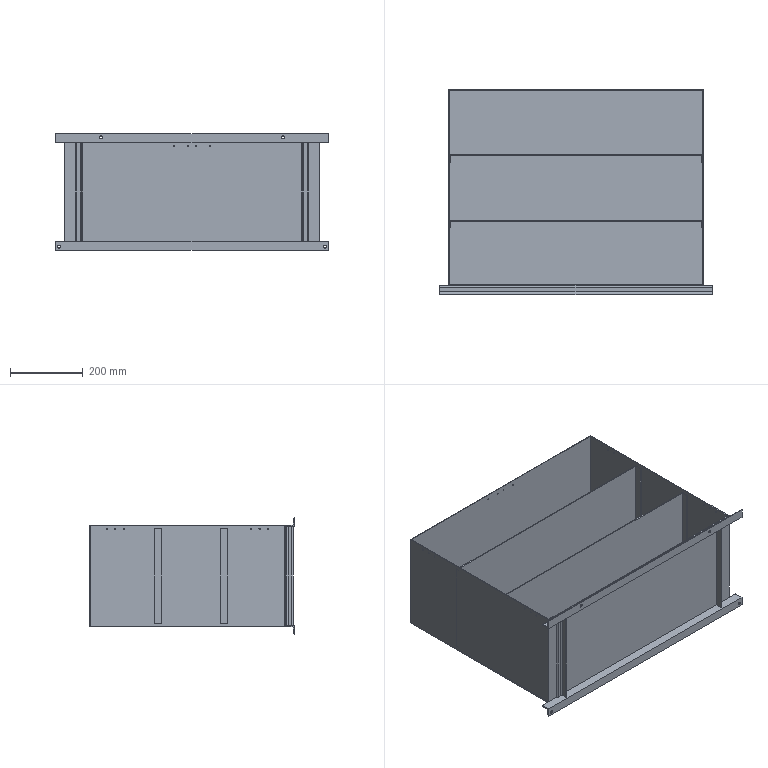Part | STEP file | OP10-009_shelf(Default_As Machined_) | 7 solids | 115 faces | box 750 x 565 x 320 mm | volume 3649347 mm3 | cylinder 60 | plane 55 | commonest cylinder face diameters 3.3 x24 2.5 x16 8 x12 6 x4 7 x4